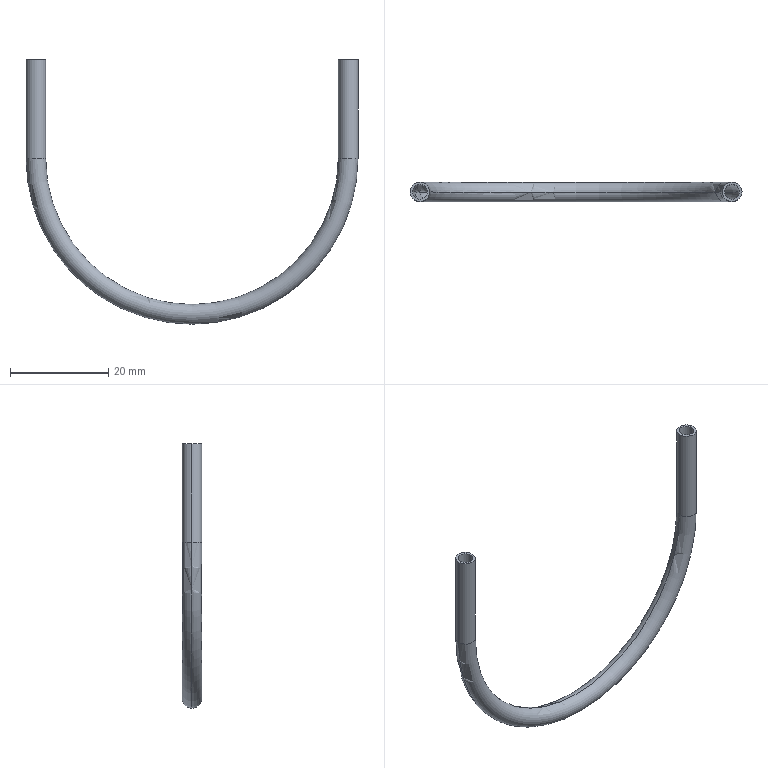Part | STEP file | 1 solid | 14 faces | box 67.5 x 4 x 53.75 mm | volume 768.291 mm3 | cylinder 8 | torus 4 | plane 2 | commonest cylinder face diameters 3 x4 4 x4
STEP:
#1=CARTESIAN_POINT('',(0.,0.,0.));
#2=DIRECTION('',(0.,0.,1.));
#3=DIRECTION('',(1.,0.,0.));
#4=AXIS2_PLACEMENT_3D('',#1,#2,#3);
#5=CARTESIAN_POINT('',(33.75,0.,0.));
#6=VERTEX_POINT('',#5);
#7=CARTESIAN_POINT('',(33.75,0.,-20.));
#8=VERTEX_POINT('',#7);
#9=CARTESIAN_POINT('',(33.75,0.,0.));
#10=DIRECTION('',(0.,0.,-1.));
#11=VECTOR('',#10,1.);
#12=LINE('',#9,#11);
#13=CARTESIAN_POINT('',(31.75,0.,0.));
#14=DIRECTION('',(0.,0.,-1.));
#15=DIRECTION('',(-1.,0.,0.));
#16=AXIS2_PLACEMENT_3D('',#13,#14,#15);
#17=CYLINDRICAL_SURFACE('',#16,2.);
#18=CARTESIAN_POINT('',(3.142,0.));
#19=DIRECTION('',(0.,1.));
#20=VECTOR('',#19,1.);
#21=LINE('',#18,#20);
#22=(GEOMETRIC_REPRESENTATION_CONTEXT(2)PARAMETRIC_REPRESENTATION_CONTEXT()REPRESENTATION_CONTEXT('',''));
#23=DEFINITIONAL_REPRESENTATION('',(#21),#22);
#24=PCURVE('',#17,#23);
#25=CARTESIAN_POINT('',(31.75,0.,0.));
#26=DIRECTION('',(0.,0.,-1.));
#27=DIRECTION('',(-1.,0.,0.));
#28=AXIS2_PLACEMENT_3D('',#25,#26,#27);
#29=CYLINDRICAL_SURFACE('',#28,2.);
#30=CARTESIAN_POINT('',(3.142,0.));
#31=DIRECTION('',(0.,1.));
#32=VECTOR('',#31,1.);
#33=LINE('',#30,#32);
#34=(GEOMETRIC_REPRESENTATION_CONTEXT(2)PARAMETRIC_REPRESENTATION_CONTEXT()REPRESENTATION_CONTEXT('',''));
#35=DEFINITIONAL_REPRESENTATION('',(#33),#34);
#36=PCURVE('',#29,#35);
#37=SURFACE_CURVE('',#12,(#24,#36),.PCURVE_S1.);
#38=EDGE_CURVE('',#6,#8,#37,.T.);
#39=ORIENTED_EDGE('',*,*,#38,.F.);
#40=CARTESIAN_POINT('',(29.75,0.,0.));
#41=VERTEX_POINT('',#40);
#42=CARTESIAN_POINT('',(31.75,0.,0.));
#43=DIRECTION('',(0.,0.,-1.));
#44=DIRECTION('',(-1.,0.,0.));
#45=AXIS2_PLACEMENT_3D('',#42,#43,#44);
#46=CIRCLE('',#45,2.);
#47=CARTESIAN_POINT('',(0.,0.));
#48=DIRECTION('',(1.,0.));
#49=VECTOR('',#48,1.);
#50=LINE('',#47,#49);
#51=(GEOMETRIC_REPRESENTATION_CONTEXT(2)PARAMETRIC_REPRESENTATION_CONTEXT()REPRESENTATION_CONTEXT('',''));
#52=DEFINITIONAL_REPRESENTATION('',(#50),#51);
#53=PCURVE('',#17,#52);
#54=CARTESIAN_POINT('',(31.75,0.,0.));
#55=DIRECTION('',(0.,0.,-1.));
#56=DIRECTION('',(-1.,0.,0.));
#57=AXIS2_PLACEMENT_3D('',#54,#55,#56);
#58=PLANE('',#57);
#59=CARTESIAN_POINT('',(0.,0.));
#60=DIRECTION('',(1.,0.));
#61=AXIS2_PLACEMENT_2D('',#59,#60);
#62=CIRCLE('',#61,2.);
#63=(GEOMETRIC_REPRESENTATION_CONTEXT(2)PARAMETRIC_REPRESENTATION_CONTEXT()REPRESENTATION_CONTEXT('',''));
#64=DEFINITIONAL_REPRESENTATION('',(#62),#63);
#65=PCURVE('',#58,#64);
#66=SURFACE_CURVE('',#46,(#53,#65),.PCURVE_S1.);
#67=EDGE_CURVE('',#6,#41,#66,.T.);
#68=ORIENTED_EDGE('',*,*,#67,.T.);
#69=CARTESIAN_POINT('',(29.75,0.,-20.));
#70=VERTEX_POINT('',#69);
#71=CARTESIAN_POINT('',(29.75,0.,0.));
#72=DIRECTION('',(0.,0.,-1.));
#73=VECTOR('',#72,1.);
#74=LINE('',#71,#73);
#75=CARTESIAN_POINT('',(6.283,0.));
#76=DIRECTION('',(0.,1.));
#77=VECTOR('',#76,1.);
#78=LINE('',#75,#77);
#79=(GEOMETRIC_REPRESENTATION_CONTEXT(2)PARAMETRIC_REPRESENTATION_CONTEXT()REPRESENTATION_CONTEXT('',''));
#80=DEFINITIONAL_REPRESENTATION('',(#78),#79);
#81=PCURVE('',#17,#80);
#82=CARTESIAN_POINT('',(0.,0.));
#83=DIRECTION('',(0.,1.));
#84=VECTOR('',#83,1.);
#85=LINE('',#82,#84);
#86=(GEOMETRIC_REPRESENTATION_CONTEXT(2)PARAMETRIC_REPRESENTATION_CONTEXT()REPRESENTATION_CONTEXT('',''));
#87=DEFINITIONAL_REPRESENTATION('',(#85),#86);
#88=PCURVE('',#29,#87);
#89=SURFACE_CURVE('',#74,(#81,#88),.PCURVE_S1.);
#90=EDGE_CURVE('',#41,#70,#89,.T.);
#91=ORIENTED_EDGE('',*,*,#90,.T.);
#92=CARTESIAN_POINT('',(31.75,0.,-20.));
#93=DIRECTION('',(0.,0.,-1.));
#94=DIRECTION('',(-1.,0.,0.));
#95=AXIS2_PLACEMENT_3D('',#92,#93,#94);
#96=CIRCLE('',#95,2.);
#97=CARTESIAN_POINT('',(0.,20.));
#98=DIRECTION('',(1.,0.));
#99=VECTOR('',#98,1.);
#100=LINE('',#97,#99);
#101=(GEOMETRIC_REPRESENTATION_CONTEXT(2)PARAMETRIC_REPRESENTATION_CONTEXT()REPRESENTATION_CONTEXT('',''));
#102=DEFINITIONAL_REPRESENTATION('',(#100),#101);
#103=PCURVE('',#17,#102);
#104=CARTESIAN_POINT('',(0.,0.,-20.));
#105=DIRECTION('',(0.,1.,0.));
#106=DIRECTION('',(0.,0.,1.));
#107=AXIS2_PLACEMENT_3D('',#104,#105,#106);
#108=TOROIDAL_SURFACE('',#107,31.75,2.);
#109=CARTESIAN_POINT('',(1.571,9.425));
#110=DIRECTION('',(0.,-1.));
#111=VECTOR('',#110,1.);
#112=LINE('',#109,#111);
#113=(GEOMETRIC_REPRESENTATION_CONTEXT(2)PARAMETRIC_REPRESENTATION_CONTEXT()REPRESENTATION_CONTEXT('',''));
#114=DEFINITIONAL_REPRESENTATION('',(#112),#113);
#115=PCURVE('',#108,#114);
#116=SURFACE_CURVE('',#96,(#103,#115),.PCURVE_S1.);
#117=EDGE_CURVE('',#8,#70,#116,.T.);
#118=ORIENTED_EDGE('',*,*,#117,.F.);
#119=EDGE_LOOP('',(#39,#68,#91,#118));
#120=FACE_BOUND('',#119,.T.);
#121=ADVANCED_FACE('',(#120),#17,.T.);
#122=CARTESIAN_POINT('',(-33.75,0.,-20.));
#123=VERTEX_POINT('',#122);
#124=CARTESIAN_POINT('',(0.,0.,-20.));
#125=DIRECTION('',(0.,1.,0.));
#126=DIRECTION('',(0.,0.,1.));
#127=AXIS2_PLACEMENT_3D('',#124,#125,#126);
#128=CIRCLE('',#127,33.75);
#129=CARTESIAN_POINT('',(0.,6.283));
#130=DIRECTION('',(1.,0.));
#131=VECTOR('',#130,1.);
#132=LINE('',#129,#131);
#133=(GEOMETRIC_REPRESENTATION_CONTEXT(2)PARAMETRIC_REPRESENTATION_CONTEXT()REPRESENTATION_CONTEXT('',''));
#134=DEFINITIONAL_REPRESENTATION('',(#132),#133);
#135=PCURVE('',#108,#134);
#136=CARTESIAN_POINT('',(0.,0.,-20.));
#137=DIRECTION('',(0.,1.,0.));
#138=DIRECTION('',(0.,0.,1.));
#139=AXIS2_PLACEMENT_3D('',#136,#137,#138);
#140=TOROIDAL_SURFACE('',#139,31.75,2.);
#141=CARTESIAN_POINT('',(0.,0.));
#142=DIRECTION('',(1.,0.));
#143=VECTOR('',#142,1.);
#144=LINE('',#141,#143);
#145=(GEOMETRIC_REPRESENTATION_CONTEXT(2)PARAMETRIC_REPRESENTATION_CONTEXT()REPRESENTATION_CONTEXT('',''));
#146=DEFINITIONAL_REPRESENTATION('',(#144),#145);
#147=PCURVE('',#140,#146);
#148=SURFACE_CURVE('',#128,(#135,#147),.PCURVE_S1.);
#149=EDGE_CURVE('',#8,#123,#148,.T.);
#150=ORIENTED_EDGE('',*,*,#149,.F.);
#151=ORIENTED_EDGE('',*,*,#117,.T.);
#152=CARTESIAN_POINT('',(-29.75,0.,-20.));
#153=VERTEX_POINT('',#152);
#154=CARTESIAN_POINT('',(0.,0.,-20.));
#155=DIRECTION('',(0.,1.,0.));
#156=DIRECTION('',(0.,0.,1.));
#157=AXIS2_PLACEMENT_3D('',#154,#155,#156);
#158=CIRCLE('',#157,29.75);
#159=CARTESIAN_POINT('',(0.,3.142));
#160=DIRECTION('',(1.,0.));
#161=VECTOR('',#160,1.);
#162=LINE('',#159,#161);
#163=(GEOMETRIC_REPRESENTATION_CONTEXT(2)PARAMETRIC_REPRESENTATION_CONTEXT()REPRESENTATION_CONTEXT('',''));
#164=DEFINITIONAL_REPRESENTATION('',(#162),#163);
#165=PCURVE('',#108,#164);
#166=CARTESIAN_POINT('',(0.,3.142));
#167=DIRECTION('',(1.,0.));
#168=VECTOR('',#167,1.);
#169=LINE('',#166,#168);
#170=(GEOMETRIC_REPRESENTATION_CONTEXT(2)PARAMETRIC_REPRESENTATION_CONTEXT()REPRESENTATION_CONTEXT('',''));
#171=DEFINITIONAL_REPRESENTATION('',(#169),#170);
#172=PCURVE('',#140,#171);
#173=SURFACE_CURVE('',#158,(#165,#172),.PCURVE_S1.);
#174=EDGE_CURVE('',#70,#153,#173,.T.);
#175=ORIENTED_EDGE('',*,*,#174,.T.);
#176=CARTESIAN_POINT('',(-31.75,0.,-20.));
#177=DIRECTION('',(0.,0.,1.));
#178=DIRECTION('',(1.,0.,0.));
#179=AXIS2_PLACEMENT_3D('',#176,#177,#178);
#180=CIRCLE('',#179,2.);
#181=CARTESIAN_POINT('',(4.712,9.425));
#182=DIRECTION('',(0.,-1.));
#183=VECTOR('',#182,1.);
#184=LINE('',#181,#183);
#185=(GEOMETRIC_REPRESENTATION_CONTEXT(2)PARAMETRIC_REPRESENTATION_CONTEXT()REPRESENTATION_CONTEXT('',''));
#186=DEFINITIONAL_REPRESENTATION('',(#184),#185);
#187=PCURVE('',#108,#186);
#188=CARTESIAN_POINT('',(-31.75,0.,-20.));
#189=DIRECTION('',(0.,0.,1.));
#190=DIRECTION('',(1.,0.,0.));
#191=AXIS2_PLACEMENT_3D('',#188,#189,#190);
#192=CYLINDRICAL_SURFACE('',#191,2.);
#193=CARTESIAN_POINT('',(0.,0.));
#194=DIRECTION('',(1.,0.));
#195=VECTOR('',#194,1.);
#196=LINE('',#193,#195);
#197=(GEOMETRIC_REPRESENTATION_CONTEXT(2)PARAMETRIC_REPRESENTATION_CONTEXT()REPRESENTATION_CONTEXT('',''));
#198=DEFINITIONAL_REPRESENTATION('',(#196),#197);
#199=PCURVE('',#192,#198);
#200=SURFACE_CURVE('',#180,(#187,#199),.PCURVE_S1.);
#201=EDGE_CURVE('',#123,#153,#200,.T.);
#202=ORIENTED_EDGE('',*,*,#201,.F.);
#203=EDGE_LOOP('',(#150,#151,#175,#202));
#204=FACE_BOUND('',#203,.T.);
#205=ADVANCED_FACE('',(#204),#108,.T.);
#206=CARTESIAN_POINT('',(-33.75,0.,0.));
#207=VERTEX_POINT('',#206);
#208=CARTESIAN_POINT('',(-33.75,0.,-20.));
#209=DIRECTION('',(0.,0.,1.));
#210=VECTOR('',#209,1.);
#211=LINE('',#208,#210);
#212=CARTESIAN_POINT('',(3.142,0.));
#213=DIRECTION('',(0.,1.));
#214=VECTOR('',#213,1.);
#215=LINE('',#212,#214);
#216=(GEOMETRIC_REPRESENTATION_CONTEXT(2)PARAMETRIC_REPRESENTATION_CONTEXT()REPRESENTATION_CONTEXT('',''));
#217=DEFINITIONAL_REPRESENTATION('',(#215),#216);
#218=PCURVE('',#192,#217);
#219=CARTESIAN_POINT('',(-31.75,0.,-20.));
#220=DIRECTION('',(0.,0.,1.));
#221=DIRECTION('',(1.,0.,0.));
#222=AXIS2_PLACEMENT_3D('',#219,#220,#221);
#223=CYLINDRICAL_SURFACE('',#222,2.);
#224=CARTESIAN_POINT('',(3.142,0.));
#225=DIRECTION('',(0.,1.));
#226=VECTOR('',#225,1.);
#227=LINE('',#224,#226);
#228=(GEOMETRIC_REPRESENTATION_CONTEXT(2)PARAMETRIC_REPRESENTATION_CONTEXT()REPRESENTATION_CONTEXT('',''));
#229=DEFINITIONAL_REPRESENTATION('',(#227),#228);
#230=PCURVE('',#223,#229);
#231=SURFACE_CURVE('',#211,(#218,#230),.PCURVE_S1.);
#232=EDGE_CURVE('',#123,#207,#231,.T.);
#233=ORIENTED_EDGE('',*,*,#232,.F.);
#234=ORIENTED_EDGE('',*,*,#201,.T.);
#235=CARTESIAN_POINT('',(-29.75,0.,0.));
#236=VERTEX_POINT('',#235);
#237=CARTESIAN_POINT('',(-29.75,0.,-20.));
#238=DIRECTION('',(0.,0.,1.));
#239=VECTOR('',#238,1.);
#240=LINE('',#237,#239);
#241=CARTESIAN_POINT('',(6.283,0.));
#242=DIRECTION('',(0.,1.));
#243=VECTOR('',#242,1.);
#244=LINE('',#241,#243);
#245=(GEOMETRIC_REPRESENTATION_CONTEXT(2)PARAMETRIC_REPRESENTATION_CONTEXT()REPRESENTATION_CONTEXT('',''));
#246=DEFINITIONAL_REPRESENTATION('',(#244),#245);
#247=PCURVE('',#192,#246);
#248=CARTESIAN_POINT('',(0.,0.));
#249=DIRECTION('',(0.,1.));
#250=VECTOR('',#249,1.);
#251=LINE('',#248,#250);
#252=(GEOMETRIC_REPRESENTATION_CONTEXT(2)PARAMETRIC_REPRESENTATION_CONTEXT()REPRESENTATION_CONTEXT('',''));
#253=DEFINITIONAL_REPRESENTATION('',(#251),#252);
#254=PCURVE('',#223,#253);
#255=SURFACE_CURVE('',#240,(#247,#254),.PCURVE_S1.);
#256=EDGE_CURVE('',#153,#236,#255,.T.);
#257=ORIENTED_EDGE('',*,*,#256,.T.);
#258=CARTESIAN_POINT('',(-31.75,0.,0.));
#259=DIRECTION('',(0.,0.,1.));
#260=DIRECTION('',(1.,0.,0.));
#261=AXIS2_PLACEMENT_3D('',#258,#259,#260);
#262=CIRCLE('',#261,2.);
#263=CARTESIAN_POINT('',(0.,20.));
#264=DIRECTION('',(1.,0.));
#265=VECTOR('',#264,1.);
#266=LINE('',#263,#265);
#267=(GEOMETRIC_REPRESENTATION_CONTEXT(2)PARAMETRIC_REPRESENTATION_CONTEXT()REPRESENTATION_CONTEXT('',''));
#268=DEFINITIONAL_REPRESENTATION('',(#266),#267);
#269=PCURVE('',#192,#268);
#270=CARTESIAN_POINT('',(-31.75,0.,0.));
#271=DIRECTION('',(0.,0.,1.));
#272=DIRECTION('',(1.,0.,0.));
#273=AXIS2_PLACEMENT_3D('',#270,#271,#272);
#274=PLANE('',#273);
#275=CARTESIAN_POINT('',(0.,0.));
#276=DIRECTION('',(1.,0.));
#277=AXIS2_PLACEMENT_2D('',#275,#276);
#278=CIRCLE('',#277,2.);
#279=(GEOMETRIC_REPRESENTATION_CONTEXT(2)PARAMETRIC_REPRESENTATION_CONTEXT()REPRESENTATION_CONTEXT('',''));
#280=DEFINITIONAL_REPRESENTATION('',(#278),#279);
#281=PCURVE('',#274,#280);
#282=SURFACE_CURVE('',#262,(#269,#281),.PCURVE_S1.);
#283=EDGE_CURVE('',#207,#236,#282,.T.);
#284=ORIENTED_EDGE('',*,*,#283,.F.);
#285=EDGE_LOOP('',(#233,#234,#257,#284));
#286=FACE_BOUND('',#285,.T.);
#287=ADVANCED_FACE('',(#286),#192,.T.);
#288=CARTESIAN_POINT('',(31.75,0.,0.));
#289=DIRECTION('',(0.,0.,-1.));
#290=DIRECTION('',(-1.,0.,0.));
#291=AXIS2_PLACEMENT_3D('',#288,#289,#290);
#292=CIRCLE('',#291,2.);
#293=CARTESIAN_POINT('',(0.,0.));
#294=DIRECTION('',(1.,0.));
#295=AXIS2_PLACEMENT_2D('',#293,#294);
#296=CIRCLE('',#295,2.);
#297=(GEOMETRIC_REPRESENTATION_CONTEXT(2)PARAMETRIC_REPRESENTATION_CONTEXT()REPRESENTATION_CONTEXT('',''));
#298=DEFINITIONAL_REPRESENTATION('',(#296),#297);
#299=PCURVE('',#58,#298);
#300=CARTESIAN_POINT('',(0.,0.));
#301=DIRECTION('',(1.,0.));
#302=VECTOR('',#301,1.);
#303=LINE('',#300,#302);
#304=(GEOMETRIC_REPRESENTATION_CONTEXT(2)PARAMETRIC_REPRESENTATION_CONTEXT()REPRESENTATION_CONTEXT('',''));
#305=DEFINITIONAL_REPRESENTATION('',(#303),#304);
#306=PCURVE('',#29,#305);
#307=SURFACE_CURVE('',#292,(#299,#306),.PCURVE_S1.);
#308=EDGE_CURVE('',#41,#6,#307,.T.);
#309=ORIENTED_EDGE('',*,*,#308,.F.);
#310=ORIENTED_EDGE('',*,*,#67,.F.);
#311=EDGE_LOOP('',(#309,#310));
#312=FACE_BOUND('',#311,.T.);
#313=CARTESIAN_POINT('',(30.25,0.,0.));
#314=VERTEX_POINT('',#313);
#315=CARTESIAN_POINT('',(33.25,0.,0.));
#316=VERTEX_POINT('',#315);
#317=CARTESIAN_POINT('',(31.75,0.,0.));
#318=DIRECTION('',(0.,0.,1.));
#319=DIRECTION('',(-1.,0.,0.));
#320=AXIS2_PLACEMENT_3D('',#317,#318,#319);
#321=CIRCLE('',#320,1.5);
#322=CARTESIAN_POINT('',(1.5,0.));
#323=CARTESIAN_POINT('',(1.5,-2.598));
#324=CARTESIAN_POINT('',(-0.75,-1.299));
#325=CARTESIAN_POINT('',(-3.,0.));
#326=CARTESIAN_POINT('',(-0.75,1.299));
#327=CARTESIAN_POINT('',(1.5,2.598));
#328=CARTESIAN_POINT('',(1.5,0.));
#329=(BOUNDED_CURVE()B_SPLINE_CURVE(2,(#322,#323,#324,#325,#326,#327,#328),.UNSPECIFIED.,.T.,.F.)B_SPLINE_CURVE_WITH_KNOTS((1,2,2,2,2,1),(-2.094,0.,2.094,4.189,6.283,8.378),.UNSPECIFIED.)CURVE()GEOMETRIC_REPRESENTATION_ITEM()RATIONAL_B_SPLINE_CURVE((1.,0.5,1.,0.5,1.,0.5,1.))REPRESENTATION_ITEM(''));
#330=(GEOMETRIC_REPRESENTATION_CONTEXT(2)PARAMETRIC_REPRESENTATION_CONTEXT()REPRESENTATION_CONTEXT('',''));
#331=DEFINITIONAL_REPRESENTATION('',(#329),#330);
#332=PCURVE('',#58,#331);
#333=CARTESIAN_POINT('',(31.75,0.,0.));
#334=DIRECTION('',(0.,0.,-1.));
#335=DIRECTION('',(-1.,0.,0.));
#336=AXIS2_PLACEMENT_3D('',#333,#334,#335);
#337=CYLINDRICAL_SURFACE('',#336,1.5);
#338=CARTESIAN_POINT('',(6.283,0.));
#339=DIRECTION('',(-1.,0.));
#340=VECTOR('',#339,1.);
#341=LINE('',#338,#340);
#342=(GEOMETRIC_REPRESENTATION_CONTEXT(2)PARAMETRIC_REPRESENTATION_CONTEXT()REPRESENTATION_CONTEXT('',''));
#343=DEFINITIONAL_REPRESENTATION('',(#341),#342);
#344=PCURVE('',#337,#343);
#345=SURFACE_CURVE('',#321,(#332,#344),.PCURVE_S1.);
#346=EDGE_CURVE('',#314,#316,#345,.T.);
#347=ORIENTED_EDGE('',*,*,#346,.F.);
#348=CARTESIAN_POINT('',(31.75,0.,0.));
#349=DIRECTION('',(0.,0.,1.));
#350=DIRECTION('',(-1.,0.,0.));
#351=AXIS2_PLACEMENT_3D('',#348,#349,#350);
#352=CIRCLE('',#351,1.5);
#353=CARTESIAN_POINT('',(1.5,0.));
#354=CARTESIAN_POINT('',(1.5,-2.598));
#355=CARTESIAN_POINT('',(-0.75,-1.299));
#356=CARTESIAN_POINT('',(-3.,0.));
#357=CARTESIAN_POINT('',(-0.75,1.299));
#358=CARTESIAN_POINT('',(1.5,2.598));
#359=CARTESIAN_POINT('',(1.5,0.));
#360=(BOUNDED_CURVE()B_SPLINE_CURVE(2,(#353,#354,#355,#356,#357,#358,#359),.UNSPECIFIED.,.T.,.F.)B_SPLINE_CURVE_WITH_KNOTS((1,2,2,2,2,1),(-2.094,0.,2.094,4.189,6.283,8.378),.UNSPECIFIED.)CURVE()GEOMETRIC_REPRESENTATION_ITEM()RATIONAL_B_SPLINE_CURVE((1.,0.5,1.,0.5,1.,0.5,1.))REPRESENTATION_ITEM(''));
#361=(GEOMETRIC_REPRESENTATION_CONTEXT(2)PARAMETRIC_REPRESENTATION_CONTEXT()REPRESENTATION_CONTEXT('',''));
#362=DEFINITIONAL_REPRESENTATION('',(#360),#361);
#363=PCURVE('',#58,#362);
#364=CARTESIAN_POINT('',(31.75,0.,0.));
#365=DIRECTION('',(0.,0.,-1.));
#366=DIRECTION('',(-1.,0.,0.));
#367=AXIS2_PLACEMENT_3D('',#364,#365,#366);
#368=CYLINDRICAL_SURFACE('',#367,1.5);
#369=CARTESIAN_POINT('',(6.283,0.));
#370=DIRECTION('',(-1.,0.));
#371=VECTOR('',#370,1.);
#372=LINE('',#369,#371);
#373=(GEOMETRIC_REPRESENTATION_CONTEXT(2)PARAMETRIC_REPRESENTATION_CONTEXT()REPRESENTATION_CONTEXT('',''));
#374=DEFINITIONAL_REPRESENTATION('',(#372),#373);
#375=PCURVE('',#368,#374);
#376=SURFACE_CURVE('',#352,(#363,#375),.PCURVE_S1.);
#377=EDGE_CURVE('',#316,#314,#376,.T.);
#378=ORIENTED_EDGE('',*,*,#377,.F.);
#379=EDGE_LOOP('',(#347,#378));
#380=FACE_BOUND('',#379,.T.);
#381=ADVANCED_FACE('',(#312,#380),#58,.F.);
#382=CARTESIAN_POINT('',(-31.75,0.,0.));
#383=DIRECTION('',(0.,0.,1.));
#384=DIRECTION('',(1.,0.,0.));
#385=AXIS2_PLACEMENT_3D('',#382,#383,#384);
#386=CIRCLE('',#385,2.);
#387=CARTESIAN_POINT('',(0.,0.));
#388=DIRECTION('',(1.,0.));
#389=AXIS2_PLACEMENT_2D('',#387,#388);
#390=CIRCLE('',#389,2.);
#391=(GEOMETRIC_REPRESENTATION_CONTEXT(2)PARAMETRIC_REPRESENTATION_CONTEXT()REPRESENTATION_CONTEXT('',''));
#392=DEFINITIONAL_REPRESENTATION('',(#390),#391);
#393=PCURVE('',#274,#392);
#394=CARTESIAN_POINT('',(0.,20.));
#395=DIRECTION('',(1.,0.));
#396=VECTOR('',#395,1.);
#397=LINE('',#394,#396);
#398=(GEOMETRIC_REPRESENTATION_CONTEXT(2)PARAMETRIC_REPRESENTATION_CONTEXT()REPRESENTATION_CONTEXT('',''));
#399=DEFINITIONAL_REPRESENTATION('',(#397),#398);
#400=PCURVE('',#223,#399);
#401=SURFACE_CURVE('',#386,(#393,#400),.PCURVE_S1.);
#402=EDGE_CURVE('',#236,#207,#401,.T.);
#403=ORIENTED_EDGE('',*,*,#402,.T.);
#404=ORIENTED_EDGE('',*,*,#283,.T.);
#405=EDGE_LOOP('',(#403,#404));
#406=FACE_BOUND('',#405,.T.);
#407=CARTESIAN_POINT('',(-30.25,0.,0.));
#408=VERTEX_POINT('',#407);
#409=CARTESIAN_POINT('',(-33.25,0.,0.));
#410=VERTEX_POINT('',#409);
#411=CARTESIAN_POINT('',(-31.75,0.,0.));
#412=DIRECTION('',(0.,0.,-1.));
#413=DIRECTION('',(1.,0.,0.));
#414=AXIS2_PLACEMENT_3D('',#411,#412,#413);
#415=CIRCLE('',#414,1.5);
#416=CARTESIAN_POINT('',(1.5,0.));
#417=CARTESIAN_POINT('',(1.5,-2.598));
#418=CARTESIAN_POINT('',(-0.75,-1.299));
#419=CARTESIAN_POINT('',(-3.,0.));
#420=CARTESIAN_POINT('',(-0.75,1.299));
#421=CARTESIAN_POINT('',(1.5,2.598));
#422=CARTESIAN_POINT('',(1.5,0.));
#423=(BOUNDED_CURVE()B_SPLINE_CURVE(2,(#416,#417,#418,#419,#420,#421,#422),.UNSPECIFIED.,.T.,.F.)B_SPLINE_CURVE_WITH_KNOTS((1,2,2,2,2,1),(-2.094,0.,2.094,4.189,6.283,8.378),.UNSPECIFIED.)CURVE()GEOMETRIC_REPRESENTATION_ITEM()RATIONAL_B_SPLINE_CURVE((1.,0.5,1.,0.5,1.,0.5,1.))REPRESENTATION_ITEM(''));
#424=(GEOMETRIC_REPRESENTATION_CONTEXT(2)PARAMETRIC_REPRESENTATION_CONTEXT()REPRESENTATION_CONTEXT('',''));
#425=DEFINITIONAL_REPRESENTATION('',(#423),#424);
#426=PCURVE('',#274,#425);
#427=CARTESIAN_POINT('',(-31.75,0.,-20.));
#428=DIRECTION('',(0.,0.,1.));
#429=DIRECTION('',(1.,0.,0.));
#430=AXIS2_PLACEMENT_3D('',#427,#428,#429);
#431=CYLINDRICAL_SURFACE('',#430,1.5);
#432=CARTESIAN_POINT('',(6.283,20.));
#433=DIRECTION('',(-1.,0.));
#434=VECTOR('',#433,1.);
#435=LINE('',#432,#434);
#436=(GEOMETRIC_REPRESENTATION_CONTEXT(2)PARAMETRIC_REPRESENTATION_CONTEXT()REPRESENTATION_CONTEXT('',''));
#437=DEFINITIONAL_REPRESENTATION('',(#435),#436);
#438=PCURVE('',#431,#437);
#439=SURFACE_CURVE('',#415,(#426,#438),.PCURVE_S1.);
#440=EDGE_CURVE('',#408,#410,#439,.T.);
#441=ORIENTED_EDGE('',*,*,#440,.T.);
#442=CARTESIAN_POINT('',(-31.75,0.,0.));
#443=DIRECTION('',(0.,0.,-1.));
#444=DIRECTION('',(1.,0.,0.));
#445=AXIS2_PLACEMENT_3D('',#442,#443,#444);
#446=CIRCLE('',#445,1.5);
#447=CARTESIAN_POINT('',(1.5,0.));
#448=CARTESIAN_POINT('',(1.5,-2.598));
#449=CARTESIAN_POINT('',(-0.75,-1.299));
#450=CARTESIAN_POINT('',(-3.,0.));
#451=CARTESIAN_POINT('',(-0.75,1.299));
#452=CARTESIAN_POINT('',(1.5,2.598));
#453=CARTESIAN_POINT('',(1.5,0.));
#454=(BOUNDED_CURVE()B_SPLINE_CURVE(2,(#447,#448,#449,#450,#451,#452,#453),.UNSPECIFIED.,.T.,.F.)B_SPLINE_CURVE_WITH_KNOTS((1,2,2,2,2,1),(-2.094,0.,2.094,4.189,6.283,8.378),.UNSPECIFIED.)CURVE()GEOMETRIC_REPRESENTATION_ITEM()RATIONAL_B_SPLINE_CURVE((1.,0.5,1.,0.5,1.,0.5,1.))REPRESENTATION_ITEM(''));
#455=(GEOMETRIC_REPRESENTATION_CONTEXT(2)PARAMETRIC_REPRESENTATION_CONTEXT()REPRESENTATION_CONTEXT('',''));
#456=DEFINITIONAL_REPRESENTATION('',(#454),#455);
#457=PCURVE('',#274,#456);
#458=CARTESIAN_POINT('',(-31.75,0.,-20.));
#459=DIRECTION('',(0.,0.,1.));
#460=DIRECTION('',(1.,0.,0.));
#461=AXIS2_PLACEMENT_3D('',#458,#459,#460);
#462=CYLINDRICAL_SURFACE('',#461,1.5);
#463=CARTESIAN_POINT('',(6.283,20.));
#464=DIRECTION('',(-1.,0.));
#465=VECTOR('',#464,1.);
#466=LINE('',#463,#465);
#467=(GEOMETRIC_REPRESENTATION_CONTEXT(2)PARAMETRIC_REPRESENTATION_CONTEXT()REPRESENTATION_CONTEXT('',''));
#468=DEFINITIONAL_REPRESENTATION('',(#466),#467);
#469=PCURVE('',#462,#468);
#470=SURFACE_CURVE('',#446,(#457,#469),.PCURVE_S1.);
#471=EDGE_CURVE('',#410,#408,#470,.T.);
#472=ORIENTED_EDGE('',*,*,#471,.T.);
#473=EDGE_LOOP('',(#441,#472));
#474=FACE_BOUND('',#473,.T.);
#475=ADVANCED_FACE('',(#406,#474),#274,.T.);
#476=CARTESIAN_POINT('',(33.25,0.,-20.));
#477=VERTEX_POINT('',#476);
#478=CARTESIAN_POINT('',(30.25,0.,-20.));
#479=VERTEX_POINT('',#478);
#480=CARTESIAN_POINT('',(31.75,0.,-20.));
#481=DIRECTION('',(0.,0.,1.));
#482=DIRECTION('',(-1.,0.,0.));
#483=AXIS2_PLACEMENT_3D('',#480,#481,#482);
#484=CIRCLE('',#483,1.5);
#485=CARTESIAN_POINT('',(6.283,20.));
#486=DIRECTION('',(-1.,0.));
#487=VECTOR('',#486,1.);
#488=LINE('',#485,#487);
#489=(GEOMETRIC_REPRESENTATION_CONTEXT(2)PARAMETRIC_REPRESENTATION_CONTEXT()REPRESENTATION_CONTEXT('',''));
#490=DEFINITIONAL_REPRESENTATION('',(#488),#489);
#491=PCURVE('',#368,#490);
#492=CARTESIAN_POINT('',(0.,0.,-20.));
#493=DIRECTION('',(0.,1.,0.));
#494=DIRECTION('',(0.,0.,1.));
#495=AXIS2_PLACEMENT_3D('',#492,#493,#494);
#496=TOROIDAL_SURFACE('',#495,31.75,1.5);
#497=CARTESIAN_POINT('',(1.571,-3.142));
#498=DIRECTION('',(0.,1.));
#499=VECTOR('',#498,1.);
#500=LINE('',#497,#499);
#501=(GEOMETRIC_REPRESENTATION_CONTEXT(2)PARAMETRIC_REPRESENTATION_CONTEXT()REPRESENTATION_CONTEXT('',''));
#502=DEFINITIONAL_REPRESENTATION('',(#500),#501);
#503=PCURVE('',#496,#502);
#504=SURFACE_CURVE('',#484,(#491,#503),.PCURVE_S1.);
#505=EDGE_CURVE('',#477,#479,#504,.T.);
#506=ORIENTED_EDGE('',*,*,#505,.T.);
#507=CARTESIAN_POINT('',(30.25,0.,0.));
#508=DIRECTION('',(0.,0.,-1.));
#509=VECTOR('',#508,1.);
#510=LINE('',#507,#509);
#511=CARTESIAN_POINT('',(0.,0.));
#512=DIRECTION('',(0.,1.));
#513=VECTOR('',#512,1.);
#514=LINE('',#511,#513);
#515=(GEOMETRIC_REPRESENTATION_CONTEXT(2)PARAMETRIC_REPRESENTATION_CONTEXT()REPRESENTATION_CONTEXT('',''));
#516=DEFINITIONAL_REPRESENTATION('',(#514),#515);
#517=PCURVE('',#368,#516);
#518=CARTESIAN_POINT('',(6.283,0.));
#519=DIRECTION('',(0.,1.));
#520=VECTOR('',#519,1.);
#521=LINE('',#518,#520);
#522=(GEOMETRIC_REPRESENTATION_CONTEXT(2)PARAMETRIC_REPRESENTATION_CONTEXT()REPRESENTATION_CONTEXT('',''));
#523=DEFINITIONAL_REPRESENTATION('',(#521),#522);
#524=PCURVE('',#337,#523);
#525=SURFACE_CURVE('',#510,(#517,#524),.PCURVE_S1.);
#526=EDGE_CURVE('',#314,#479,#525,.T.);
#527=ORIENTED_EDGE('',*,*,#526,.F.);
#528=ORIENTED_EDGE('',*,*,#377,.F.);
#529=CARTESIAN_POINT('',(33.25,0.,0.));
#530=DIRECTION('',(0.,0.,-1.));
#531=VECTOR('',#530,1.);
#532=LINE('',#529,#531);
#533=CARTESIAN_POINT('',(3.142,0.));
#534=DIRECTION('',(0.,1.));
#535=VECTOR('',#534,1.);
#536=LINE('',#533,#535);
#537=(GEOMETRIC_REPRESENTATION_CONTEXT(2)PARAMETRIC_REPRESENTATION_CONTEXT()REPRESENTATION_CONTEXT('',''));
#538=DEFINITIONAL_REPRESENTATION('',(#536),#537);
#539=PCURVE('',#368,#538);
#540=CARTESIAN_POINT('',(3.142,0.));
#541=DIRECTION('',(0.,1.));
#542=VECTOR('',#541,1.);
#543=LINE('',#540,#542);
#544=(GEOMETRIC_REPRESENTATION_CONTEXT(2)PARAMETRIC_REPRESENTATION_CONTEXT()REPRESENTATION_CONTEXT('',''));
#545=DEFINITIONAL_REPRESENTATION('',(#543),#544);
#546=PCURVE('',#337,#545);
#547=SURFACE_CURVE('',#532,(#539,#546),.PCURVE_S1.);
#548=EDGE_CURVE('',#316,#477,#547,.T.);
#549=ORIENTED_EDGE('',*,*,#548,.T.);
#550=EDGE_LOOP('',(#506,#527,#528,#549));
#551=FACE_BOUND('',#550,.F.);
#552=ADVANCED_FACE('',(#551),#368,.F.);
#553=CARTESIAN_POINT('',(-33.25,0.,-20.));
#554=VERTEX_POINT('',#553);
#555=CARTESIAN_POINT('',(-30.25,0.,-20.));
#556=VERTEX_POINT('',#555);
#557=CARTESIAN_POINT('',(-31.75,0.,-20.));
#558=DIRECTION('',(0.,0.,-1.));
#559=DIRECTION('',(1.,0.,0.));
#560=AXIS2_PLACEMENT_3D('',#557,#558,#559);
#561=CIRCLE('',#560,1.5);
#562=CARTESIAN_POINT('',(4.712,-3.142));
#563=DIRECTION('',(0.,1.));
#564=VECTOR('',#563,1.);
#565=LINE('',#562,#564);
#566=(GEOMETRIC_REPRESENTATION_CONTEXT(2)PARAMETRIC_REPRESENTATION_CONTEXT()REPRESENTATION_CONTEXT('',''));
#567=DEFINITIONAL_REPRESENTATION('',(#565),#566);
#568=PCURVE('',#496,#567);
#569=CARTESIAN_POINT('',(6.283,0.));
#570=DIRECTION('',(-1.,0.));
#571=VECTOR('',#570,1.);
#572=LINE('',#569,#571);
#573=(GEOMETRIC_REPRESENTATION_CONTEXT(2)PARAMETRIC_REPRESENTATION_CONTEXT()REPRESENTATION_CONTEXT('',''));
#574=DEFINITIONAL_REPRESENTATION('',(#572),#573);
#575=PCURVE('',#462,#574);
#576=SURFACE_CURVE('',#561,(#568,#575),.PCURVE_S1.);
#577=EDGE_CURVE('',#554,#556,#576,.T.);
#578=ORIENTED_EDGE('',*,*,#577,.T.);
#579=CARTESIAN_POINT('',(0.,0.,-20.));
#580=DIRECTION('',(0.,1.,0.));
#581=DIRECTION('',(0.,0.,1.));
#582=AXIS2_PLACEMENT_3D('',#579,#580,#581);
#583=CIRCLE('',#582,30.25);
#584=CARTESIAN_POINT('',(0.,3.142));
#585=DIRECTION('',(1.,0.));
#586=VECTOR('',#585,1.);
#587=LINE('',#584,#586);
#588=(GEOMETRIC_REPRESENTATION_CONTEXT(2)PARAMETRIC_REPRESENTATION_CONTEXT()REPRESENTATION_CONTEXT('',''));
#589=DEFINITIONAL_REPRESENTATION('',(#587),#588);
#590=PCURVE('',#496,#589);
#591=CARTESIAN_POINT('',(0.,0.,-20.));
#592=DIRECTION('',(0.,1.,0.));
#593=DIRECTION('',(0.,0.,1.));
#594=AXIS2_PLACEMENT_3D('',#591,#592,#593);
#595=TOROIDAL_SURFACE('',#594,31.75,1.5);
#596=CARTESIAN_POINT('',(0.,3.142));
#597=DIRECTION('',(1.,0.));
#598=VECTOR('',#597,1.);
#599=LINE('',#596,#598);
#600=(GEOMETRIC_REPRESENTATION_CONTEXT(2)PARAMETRIC_REPRESENTATION_CONTEXT()REPRESENTATION_CONTEXT('',''));
#601=DEFINITIONAL_REPRESENTATION('',(#599),#600);
#602=PCURVE('',#595,#601);
#603=SURFACE_CURVE('',#583,(#590,#602),.PCURVE_S1.);
#604=EDGE_CURVE('',#479,#556,#603,.T.);
#605=ORIENTED_EDGE('',*,*,#604,.F.);
#606=ORIENTED_EDGE('',*,*,#505,.F.);
#607=CARTESIAN_POINT('',(0.,0.,-20.));
#608=DIRECTION('',(0.,1.,0.));
#609=DIRECTION('',(0.,0.,1.));
#610=AXIS2_PLACEMENT_3D('',#607,#608,#609);
#611=CIRCLE('',#610,33.25);
#612=CARTESIAN_POINT('',(0.,0.));
#613=DIRECTION('',(1.,0.));
#614=VECTOR('',#613,1.);
#615=LINE('',#612,#614);
#616=(GEOMETRIC_REPRESENTATION_CONTEXT(2)PARAMETRIC_REPRESENTATION_CONTEXT()REPRESENTATION_CONTEXT('',''));
#617=DEFINITIONAL_REPRESENTATION('',(#615),#616);
#618=PCURVE('',#496,#617);
#619=CARTESIAN_POINT('',(0.,6.283));
#620=DIRECTION('',(1.,0.));
#621=VECTOR('',#620,1.);
#622=LINE('',#619,#621);
#623=(GEOMETRIC_REPRESENTATION_CONTEXT(2)PARAMETRIC_REPRESENTATION_CONTEXT()REPRESENTATION_CONTEXT('',''));
#624=DEFINITIONAL_REPRESENTATION('',(#622),#623);
#625=PCURVE('',#595,#624);
#626=SURFACE_CURVE('',#611,(#618,#625),.PCURVE_S1.);
#627=EDGE_CURVE('',#477,#554,#626,.T.);
#628=ORIENTED_EDGE('',*,*,#627,.T.);
#629=EDGE_LOOP('',(#578,#605,#606,#628));
#630=FACE_BOUND('',#629,.F.);
#631=ADVANCED_FACE('',(#630),#496,.F.);
#632=ORIENTED_EDGE('',*,*,#471,.T.);
#633=CARTESIAN_POINT('',(-30.25,0.,-20.));
#634=DIRECTION('',(0.,0.,1.));
#635=VECTOR('',#634,1.);
#636=LINE('',#633,#635);
#637=CARTESIAN_POINT('',(0.,0.));
#638=DIRECTION('',(0.,1.));
#639=VECTOR('',#638,1.);
#640=LINE('',#637,#639);
#641=(GEOMETRIC_REPRESENTATION_CONTEXT(2)PARAMETRIC_REPRESENTATION_CONTEXT()REPRESENTATION_CONTEXT('',''));
#642=DEFINITIONAL_REPRESENTATION('',(#640),#641);
#643=PCURVE('',#462,#642);
#644=CARTESIAN_POINT('',(6.283,0.));
#645=DIRECTION('',(0.,1.));
#646=VECTOR('',#645,1.);
#647=LINE('',#644,#646);
#648=(GEOMETRIC_REPRESENTATION_CONTEXT(2)PARAMETRIC_REPRESENTATION_CONTEXT()REPRESENTATION_CONTEXT('',''));
#649=DEFINITIONAL_REPRESENTATION('',(#647),#648);
#650=PCURVE('',#431,#649);
#651=SURFACE_CURVE('',#636,(#643,#650),.PCURVE_S1.);
#652=EDGE_CURVE('',#556,#408,#651,.T.);
#653=ORIENTED_EDGE('',*,*,#652,.F.);
#654=ORIENTED_EDGE('',*,*,#577,.F.);
#655=CARTESIAN_POINT('',(-33.25,0.,-20.));
#656=DIRECTION('',(0.,0.,1.));
#657=VECTOR('',#656,1.);
#658=LINE('',#655,#657);
#659=CARTESIAN_POINT('',(3.142,0.));
#660=DIRECTION('',(0.,1.));
#661=VECTOR('',#660,1.);
#662=LINE('',#659,#661);
#663=(GEOMETRIC_REPRESENTATION_CONTEXT(2)PARAMETRIC_REPRESENTATION_CONTEXT()REPRESENTATION_CONTEXT('',''));
#664=DEFINITIONAL_REPRESENTATION('',(#662),#663);
#665=PCURVE('',#462,#664);
#666=CARTESIAN_POINT('',(3.142,0.));
#667=DIRECTION('',(0.,1.));
#668=VECTOR('',#667,1.);
#669=LINE('',#666,#668);
#670=(GEOMETRIC_REPRESENTATION_CONTEXT(2)PARAMETRIC_REPRESENTATION_CONTEXT()REPRESENTATION_CONTEXT('',''));
#671=DEFINITIONAL_REPRESENTATION('',(#669),#670);
#672=PCURVE('',#431,#671);
#673=SURFACE_CURVE('',#658,(#665,#672),.PCURVE_S1.);
#674=EDGE_CURVE('',#554,#410,#673,.T.);
#675=ORIENTED_EDGE('',*,*,#674,.T.);
#676=EDGE_LOOP('',(#632,#653,#654,#675));
#677=FACE_BOUND('',#676,.F.);
#678=ADVANCED_FACE('',(#677),#462,.F.);
#679=ORIENTED_EDGE('',*,*,#308,.T.);
#680=ORIENTED_EDGE('',*,*,#38,.T.);
#681=CARTESIAN_POINT('',(31.75,0.,-20.));
#682=DIRECTION('',(0.,0.,-1.));
#683=DIRECTION('',(-1.,0.,0.));
#684=AXIS2_PLACEMENT_3D('',#681,#682,#683);
#685=CIRCLE('',#684,2.);
#686=CARTESIAN_POINT('',(0.,20.));
#687=DIRECTION('',(1.,0.));
#688=VECTOR('',#687,1.);
#689=LINE('',#686,#688);
#690=(GEOMETRIC_REPRESENTATION_CONTEXT(2)PARAMETRIC_REPRESENTATION_CONTEXT()REPRESENTATION_CONTEXT('',''));
#691=DEFINITIONAL_REPRESENTATION('',(#689),#690);
#692=PCURVE('',#29,#691);
#693=CARTESIAN_POINT('',(1.571,3.142));
#694=DIRECTION('',(0.,-1.));
#695=VECTOR('',#694,1.);
#696=LINE('',#693,#695);
#697=(GEOMETRIC_REPRESENTATION_CONTEXT(2)PARAMETRIC_REPRESENTATION_CONTEXT()REPRESENTATION_CONTEXT('',''));
#698=DEFINITIONAL_REPRESENTATION('',(#696),#697);
#699=PCURVE('',#140,#698);
#700=SURFACE_CURVE('',#685,(#692,#699),.PCURVE_S1.);
#701=EDGE_CURVE('',#70,#8,#700,.T.);
#702=ORIENTED_EDGE('',*,*,#701,.F.);
#703=ORIENTED_EDGE('',*,*,#90,.F.);
#704=EDGE_LOOP('',(#679,#680,#702,#703));
#705=FACE_BOUND('',#704,.T.);
#706=ADVANCED_FACE('',(#705),#29,.T.);
#707=CARTESIAN_POINT('',(-31.75,0.,-20.));
#708=DIRECTION('',(0.,0.,1.));
#709=DIRECTION('',(1.,0.,0.));
#710=AXIS2_PLACEMENT_3D('',#707,#708,#709);
#711=CIRCLE('',#710,2.);
#712=CARTESIAN_POINT('',(0.,0.));
#713=DIRECTION('',(1.,0.));
#714=VECTOR('',#713,1.);
#715=LINE('',#712,#714);
#716=(GEOMETRIC_REPRESENTATION_CONTEXT(2)PARAMETRIC_REPRESENTATION_CONTEXT()REPRESENTATION_CONTEXT('',''));
#717=DEFINITIONAL_REPRESENTATION('',(#715),#716);
#718=PCURVE('',#223,#717);
#719=CARTESIAN_POINT('',(4.712,3.142));
#720=DIRECTION('',(0.,-1.));
#721=VECTOR('',#720,1.);
#722=LINE('',#719,#721);
#723=(GEOMETRIC_REPRESENTATION_CONTEXT(2)PARAMETRIC_REPRESENTATION_CONTEXT()REPRESENTATION_CONTEXT('',''));
#724=DEFINITIONAL_REPRESENTATION('',(#722),#723);
#725=PCURVE('',#140,#724);
#726=SURFACE_CURVE('',#711,(#718,#725),.PCURVE_S1.);
#727=EDGE_CURVE('',#153,#123,#726,.T.);
#728=ORIENTED_EDGE('',*,*,#727,.T.);
#729=ORIENTED_EDGE('',*,*,#232,.T.);
#730=ORIENTED_EDGE('',*,*,#402,.F.);
#731=ORIENTED_EDGE('',*,*,#256,.F.);
#732=EDGE_LOOP('',(#728,#729,#730,#731));
#733=FACE_BOUND('',#732,.T.);
#734=ADVANCED_FACE('',(#733),#223,.T.);
#735=ORIENTED_EDGE('',*,*,#526,.T.);
#736=CARTESIAN_POINT('',(31.75,0.,-20.));
#737=DIRECTION('',(0.,0.,1.));
#738=DIRECTION('',(-1.,0.,0.));
#739=AXIS2_PLACEMENT_3D('',#736,#737,#738);
#740=CIRCLE('',#739,1.5);
#741=CARTESIAN_POINT('',(6.283,20.));
#742=DIRECTION('',(-1.,0.));
#743=VECTOR('',#742,1.);
#744=LINE('',#741,#743);
#745=(GEOMETRIC_REPRESENTATION_CONTEXT(2)PARAMETRIC_REPRESENTATION_CONTEXT()REPRESENTATION_CONTEXT('',''));
#746=DEFINITIONAL_REPRESENTATION('',(#744),#745);
#747=PCURVE('',#337,#746);
#748=CARTESIAN_POINT('',(1.571,3.142));
#749=DIRECTION('',(0.,1.));
#750=VECTOR('',#749,1.);
#751=LINE('',#748,#750);
#752=(GEOMETRIC_REPRESENTATION_CONTEXT(2)PARAMETRIC_REPRESENTATION_CONTEXT()REPRESENTATION_CONTEXT('',''));
#753=DEFINITIONAL_REPRESENTATION('',(#751),#752);
#754=PCURVE('',#595,#753);
#755=SURFACE_CURVE('',#740,(#747,#754),.PCURVE_S1.);
#756=EDGE_CURVE('',#479,#477,#755,.T.);
#757=ORIENTED_EDGE('',*,*,#756,.T.);
#758=ORIENTED_EDGE('',*,*,#548,.F.);
#759=ORIENTED_EDGE('',*,*,#346,.F.);
#760=EDGE_LOOP('',(#735,#757,#758,#759));
#761=FACE_BOUND('',#760,.F.);
#762=ADVANCED_FACE('',(#761),#337,.F.);
#763=ORIENTED_EDGE('',*,*,#652,.T.);
#764=ORIENTED_EDGE('',*,*,#440,.T.);
#765=ORIENTED_EDGE('',*,*,#674,.F.);
#766=CARTESIAN_POINT('',(-31.75,0.,-20.));
#767=DIRECTION('',(0.,0.,-1.));
#768=DIRECTION('',(1.,0.,0.));
#769=AXIS2_PLACEMENT_3D('',#766,#767,#768);
#770=CIRCLE('',#769,1.5);
#771=CARTESIAN_POINT('',(6.283,0.));
#772=DIRECTION('',(-1.,0.));
#773=VECTOR('',#772,1.);
#774=LINE('',#771,#773);
#775=(GEOMETRIC_REPRESENTATION_CONTEXT(2)PARAMETRIC_REPRESENTATION_CONTEXT()REPRESENTATION_CONTEXT('',''));
#776=DEFINITIONAL_REPRESENTATION('',(#774),#775);
#777=PCURVE('',#431,#776);
#778=CARTESIAN_POINT('',(4.712,3.142));
#779=DIRECTION('',(0.,1.));
#780=VECTOR('',#779,1.);
#781=LINE('',#778,#780);
#782=(GEOMETRIC_REPRESENTATION_CONTEXT(2)PARAMETRIC_REPRESENTATION_CONTEXT()REPRESENTATION_CONTEXT('',''));
#783=DEFINITIONAL_REPRESENTATION('',(#781),#782);
#784=PCURVE('',#595,#783);
#785=SURFACE_CURVE('',#770,(#777,#784),.PCURVE_S1.);
#786=EDGE_CURVE('',#556,#554,#785,.T.);
#787=ORIENTED_EDGE('',*,*,#786,.F.);
#788=EDGE_LOOP('',(#763,#764,#765,#787));
#789=FACE_BOUND('',#788,.F.);
#790=ADVANCED_FACE('',(#789),#431,.F.);
#791=ORIENTED_EDGE('',*,*,#701,.T.);
#792=ORIENTED_EDGE('',*,*,#149,.T.);
#793=ORIENTED_EDGE('',*,*,#727,.F.);
#794=ORIENTED_EDGE('',*,*,#174,.F.);
#795=EDGE_LOOP('',(#791,#792,#793,#794));
#796=FACE_BOUND('',#795,.T.);
#797=ADVANCED_FACE('',(#796),#140,.T.);
#798=ORIENTED_EDGE('',*,*,#604,.T.);
#799=ORIENTED_EDGE('',*,*,#786,.T.);
#800=ORIENTED_EDGE('',*,*,#627,.F.);
#801=ORIENTED_EDGE('',*,*,#756,.F.);
#802=EDGE_LOOP('',(#798,#799,#800,#801));
#803=FACE_BOUND('',#802,.F.);
#804=ADVANCED_FACE('',(#803),#595,.F.);
#805=CLOSED_SHELL('',(#121,#205,#287,#381,#475,#552,#631,#678,#706,#734,#762,#790,#797,#804));
#806=MANIFOLD_SOLID_BREP('',#805);
#807=(LENGTH_UNIT()NAMED_UNIT(*)SI_UNIT(.MILLI.,.METRE.));
#808=UNCERTAINTY_MEASURE_WITH_UNIT(LENGTH_MEASURE(0.0000001),#807,'','');
#809=(NAMED_UNIT(*)PLANE_ANGLE_UNIT()SI_UNIT($,.RADIAN.));
#810=(NAMED_UNIT(*)SI_UNIT($,.STERADIAN.)SOLID_ANGLE_UNIT());
#811=(GEOMETRIC_REPRESENTATION_CONTEXT(3)GLOBAL_UNCERTAINTY_ASSIGNED_CONTEXT((#808))GLOBAL_UNIT_ASSIGNED_CONTEXT((#807,#809,#810))REPRESENTATION_CONTEXT('',''));
#812=ADVANCED_BREP_SHAPE_REPRESENTATION('',(#4,#806),#811);